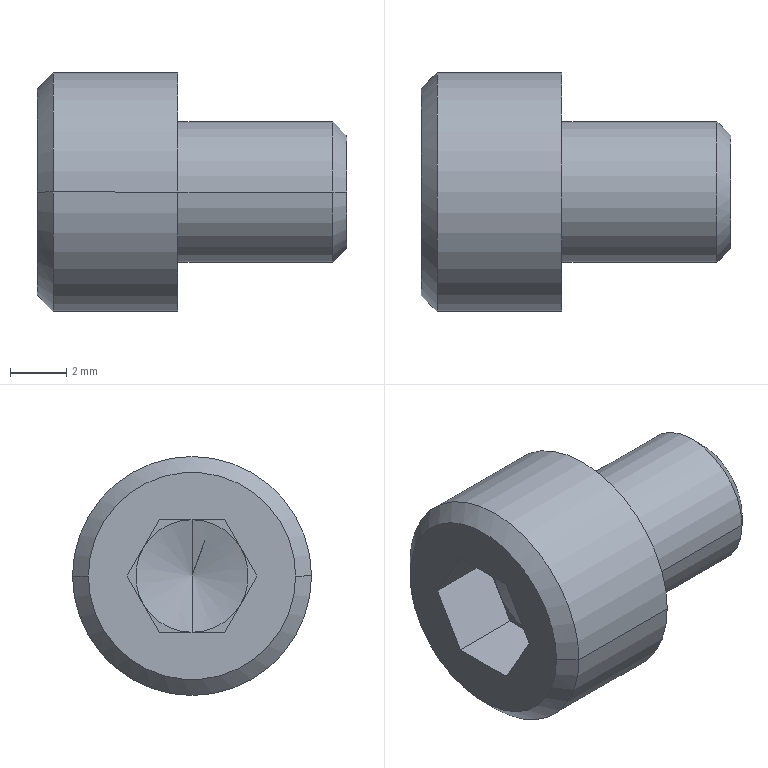Part | STEP file | CB5-6_Default | 1 solid | 25 faces | box 11 x 8.5 x 8.5 mm | volume 358.786 mm3 | plane 15 | cone 6 | cylinder 4 | commonest cylinder face diameters 5 x2 8.5 x2